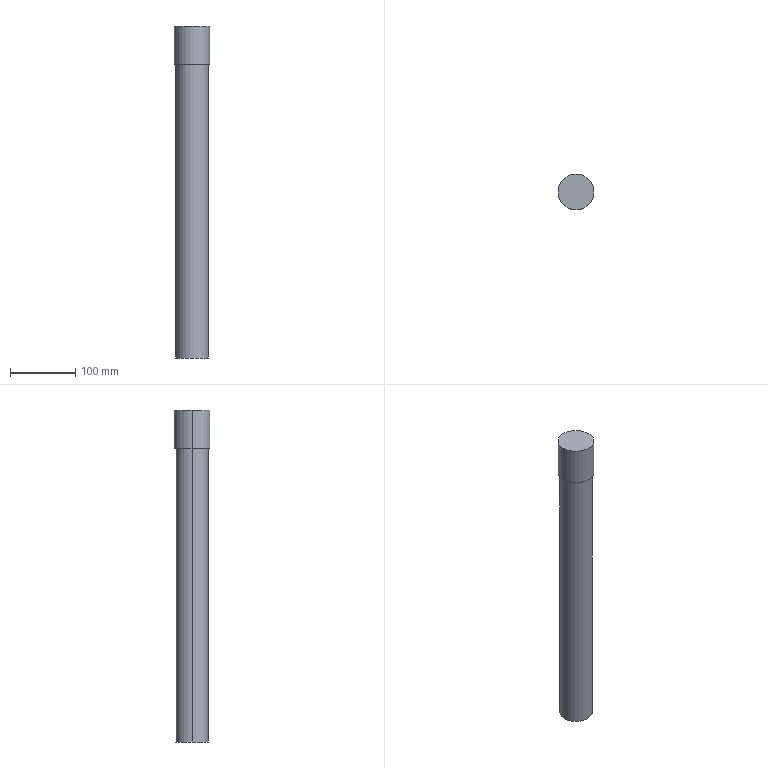Part | SolidWorks | features Extrusion 1, ICE 1 | 1 solid | 7 faces | box 55 x 55 x 509 mm | volume 1029553 mm3 | cylinder 4 | plane 3 | commonest cylinder face diameters 50.164 x2 55 x2
STEP:
#1=CARTESIAN_POINT('',(27.5,0.,59.));
#2=VERTEX_POINT('',#1);
#3=CARTESIAN_POINT('',(-27.5,0.,59.));
#4=VERTEX_POINT('',#3);
#5=CARTESIAN_POINT('',(0.,0.,59.));
#6=DIRECTION('',(0.,0.,1.));
#7=DIRECTION('',(1.,0.,0.));
#8=AXIS2_PLACEMENT_3D('',#5,#6,#7);
#9=CIRCLE('',#8,27.5);
#10=EDGE_CURVE('',#2,#4,#9,.T.);
#11=ORIENTED_EDGE('',*,*,#10,.F.);
#12=CARTESIAN_POINT('',(27.5,0.,0.));
#13=VERTEX_POINT('',#12);
#14=CARTESIAN_POINT('',(27.5,0.,136.782));
#15=DIRECTION('',(0.,0.,-1.));
#16=VECTOR('',#15,1000.);
#17=LINE('',#14,#16);
#18=EDGE_CURVE('',#2,#13,#17,.T.);
#19=ORIENTED_EDGE('',*,*,#18,.T.);
#20=CARTESIAN_POINT('',(-27.5,0.,0.));
#21=VERTEX_POINT('',#20);
#22=CARTESIAN_POINT('',(0.,0.,0.));
#23=DIRECTION('',(0.,0.,1.));
#24=DIRECTION('',(1.,0.,0.));
#25=AXIS2_PLACEMENT_3D('',#22,#23,#24);
#26=CIRCLE('',#25,27.5);
#27=EDGE_CURVE('',#13,#21,#26,.T.);
#28=ORIENTED_EDGE('',*,*,#27,.T.);
#29=CARTESIAN_POINT('',(-27.5,0.,136.782));
#30=DIRECTION('',(0.,0.,-1.));
#31=VECTOR('',#30,1000.);
#32=LINE('',#29,#31);
#33=EDGE_CURVE('',#4,#21,#32,.T.);
#34=ORIENTED_EDGE('',*,*,#33,.F.);
#35=EDGE_LOOP('',(#11,#19,#28,#34));
#36=FACE_OUTER_BOUND('',#35,.T.);
#37=CARTESIAN_POINT('',(0.,0.,136.782));
#38=DIRECTION('',(0.,0.,-1.));
#39=DIRECTION('',(-1.,0.,0.));
#40=AXIS2_PLACEMENT_3D('',#37,#38,#39);
#41=CYLINDRICAL_SURFACE('',#40,27.5);
#42=ADVANCED_FACE('',(#36),#41,.T.);
#43=CARTESIAN_POINT('',(25.082,0.,-450.));
#44=VERTEX_POINT('',#43);
#45=CARTESIAN_POINT('',(-25.082,0.,-450.));
#46=VERTEX_POINT('',#45);
#47=CARTESIAN_POINT('',(0.,0.,-450.));
#48=DIRECTION('',(0.,0.,1.));
#49=DIRECTION('',(1.,0.,0.));
#50=AXIS2_PLACEMENT_3D('',#47,#48,#49);
#51=CIRCLE('',#50,25.082);
#52=EDGE_CURVE('',#44,#46,#51,.T.);
#53=ORIENTED_EDGE('',*,*,#52,.T.);
#54=CARTESIAN_POINT('',(-25.082,0.,0.));
#55=VERTEX_POINT('',#54);
#56=CARTESIAN_POINT('',(-25.082,0.,-450.));
#57=DIRECTION('',(0.,0.,1.));
#58=VECTOR('',#57,1000.);
#59=LINE('',#56,#58);
#60=EDGE_CURVE('',#46,#55,#59,.T.);
#61=ORIENTED_EDGE('',*,*,#60,.T.);
#62=CARTESIAN_POINT('',(25.082,0.,0.));
#63=VERTEX_POINT('',#62);
#64=CARTESIAN_POINT('',(0.,0.,0.));
#65=DIRECTION('',(0.,0.,1.));
#66=DIRECTION('',(1.,0.,0.));
#67=AXIS2_PLACEMENT_3D('',#64,#65,#66);
#68=CIRCLE('',#67,25.082);
#69=EDGE_CURVE('',#63,#55,#68,.T.);
#70=ORIENTED_EDGE('',*,*,#69,.F.);
#71=CARTESIAN_POINT('',(25.082,0.,-450.));
#72=DIRECTION('',(0.,0.,1.));
#73=VECTOR('',#72,1000.);
#74=LINE('',#71,#73);
#75=EDGE_CURVE('',#44,#63,#74,.T.);
#76=ORIENTED_EDGE('',*,*,#75,.F.);
#77=EDGE_LOOP('',(#53,#61,#70,#76));
#78=FACE_OUTER_BOUND('',#77,.T.);
#79=CARTESIAN_POINT('',(0.,0.,-450.));
#80=DIRECTION('',(0.,0.,1.));
#81=DIRECTION('',(1.,0.,0.));
#82=AXIS2_PLACEMENT_3D('',#79,#80,#81);
#83=CYLINDRICAL_SURFACE('',#82,25.082);
#84=ADVANCED_FACE('',(#78),#83,.T.);
#85=ORIENTED_EDGE('',*,*,#60,.F.);
#86=CARTESIAN_POINT('',(0.,0.,-450.));
#87=DIRECTION('',(0.,0.,1.));
#88=DIRECTION('',(1.,0.,0.));
#89=AXIS2_PLACEMENT_3D('',#86,#87,#88);
#90=CIRCLE('',#89,25.082);
#91=EDGE_CURVE('',#46,#44,#90,.T.);
#92=ORIENTED_EDGE('',*,*,#91,.T.);
#93=ORIENTED_EDGE('',*,*,#75,.T.);
#94=CARTESIAN_POINT('',(0.,0.,0.));
#95=DIRECTION('',(0.,0.,1.));
#96=DIRECTION('',(1.,0.,0.));
#97=AXIS2_PLACEMENT_3D('',#94,#95,#96);
#98=CIRCLE('',#97,25.082);
#99=EDGE_CURVE('',#55,#63,#98,.T.);
#100=ORIENTED_EDGE('',*,*,#99,.F.);
#101=EDGE_LOOP('',(#85,#92,#93,#100));
#102=FACE_OUTER_BOUND('',#101,.T.);
#103=CARTESIAN_POINT('',(0.,0.,-450.));
#104=DIRECTION('',(0.,0.,1.));
#105=DIRECTION('',(1.,0.,0.));
#106=AXIS2_PLACEMENT_3D('',#103,#104,#105);
#107=CYLINDRICAL_SURFACE('',#106,25.082);
#108=ADVANCED_FACE('',(#102),#107,.T.);
#109=ORIENTED_EDGE('',*,*,#52,.F.);
#110=ORIENTED_EDGE('',*,*,#91,.F.);
#111=EDGE_LOOP('',(#109,#110));
#112=FACE_OUTER_BOUND('',#111,.T.);
#113=CARTESIAN_POINT('',(0.,0.,-450.));
#114=DIRECTION('',(0.,0.,1.));
#115=DIRECTION('',(1.,0.,0.));
#116=AXIS2_PLACEMENT_3D('',#113,#114,#115);
#117=PLANE('',#116);
#118=ADVANCED_FACE('',(#112),#117,.F.);
#119=ORIENTED_EDGE('',*,*,#18,.F.);
#120=CARTESIAN_POINT('',(0.,0.,59.));
#121=DIRECTION('',(0.,0.,1.));
#122=DIRECTION('',(1.,0.,0.));
#123=AXIS2_PLACEMENT_3D('',#120,#121,#122);
#124=CIRCLE('',#123,27.5);
#125=EDGE_CURVE('',#4,#2,#124,.T.);
#126=ORIENTED_EDGE('',*,*,#125,.F.);
#127=ORIENTED_EDGE('',*,*,#33,.T.);
#128=CARTESIAN_POINT('',(0.,0.,0.));
#129=DIRECTION('',(0.,0.,1.));
#130=DIRECTION('',(1.,0.,0.));
#131=AXIS2_PLACEMENT_3D('',#128,#129,#130);
#132=CIRCLE('',#131,27.5);
#133=EDGE_CURVE('',#21,#13,#132,.T.);
#134=ORIENTED_EDGE('',*,*,#133,.T.);
#135=EDGE_LOOP('',(#119,#126,#127,#134));
#136=FACE_OUTER_BOUND('',#135,.T.);
#137=CARTESIAN_POINT('',(0.,0.,136.782));
#138=DIRECTION('',(0.,0.,-1.));
#139=DIRECTION('',(-1.,0.,0.));
#140=AXIS2_PLACEMENT_3D('',#137,#138,#139);
#141=CYLINDRICAL_SURFACE('',#140,27.5);
#142=ADVANCED_FACE('',(#136),#141,.T.);
#143=ORIENTED_EDGE('',*,*,#69,.T.);
#144=ORIENTED_EDGE('',*,*,#99,.T.);
#145=EDGE_LOOP('',(#143,#144));
#146=FACE_BOUND('',#145,.T.);
#147=ORIENTED_EDGE('',*,*,#133,.F.);
#148=ORIENTED_EDGE('',*,*,#27,.F.);
#149=EDGE_LOOP('',(#147,#148));
#150=FACE_OUTER_BOUND('',#149,.T.);
#151=CARTESIAN_POINT('',(0.,0.,0.));
#152=DIRECTION('',(0.,0.,1.));
#153=DIRECTION('',(1.,0.,0.));
#154=AXIS2_PLACEMENT_3D('',#151,#152,#153);
#155=PLANE('',#154);
#156=ADVANCED_FACE('',(#146,#150),#155,.F.);
#157=ORIENTED_EDGE('',*,*,#125,.T.);
#158=ORIENTED_EDGE('',*,*,#10,.T.);
#159=EDGE_LOOP('',(#157,#158));
#160=FACE_OUTER_BOUND('',#159,.T.);
#161=CARTESIAN_POINT('',(0.,0.,59.));
#162=DIRECTION('',(0.,0.,1.));
#163=DIRECTION('',(-0.9989,0.0479,0.));
#164=AXIS2_PLACEMENT_3D('',#161,#162,#163);
#165=PLANE('',#164);
#166=ADVANCED_FACE('',(#160),#165,.T.);
#167=CLOSED_SHELL('',(#42,#84,#108,#118,#142,#156,#166));
#168=MANIFOLD_SOLID_BREP('',#167);
#169=CARTESIAN_POINT('',(0.,0.,0.));
#170=DIRECTION('',(0.,0.,1.));
#171=DIRECTION('',(1.,0.,0.));
#172=AXIS2_PLACEMENT_3D('',#169,#170,#171);
#173=(LENGTH_UNIT()NAMED_UNIT(*)SI_UNIT(.MILLI.,.METRE.));
#174=UNCERTAINTY_MEASURE_WITH_UNIT(LENGTH_MEASURE(0.00001),#173,'','');
#175=(NAMED_UNIT(*)PLANE_ANGLE_UNIT()SI_UNIT($,.RADIAN.));
#176=(NAMED_UNIT(*)SI_UNIT($,.STERADIAN.)SOLID_ANGLE_UNIT());
#177=(GEOMETRIC_REPRESENTATION_CONTEXT(3)GLOBAL_UNCERTAINTY_ASSIGNED_CONTEXT((#174))GLOBAL_UNIT_ASSIGNED_CONTEXT((#173,#175,#176))REPRESENTATION_CONTEXT('',''));
#178=ADVANCED_BREP_SHAPE_REPRESENTATION('',(#168,#172),#177);